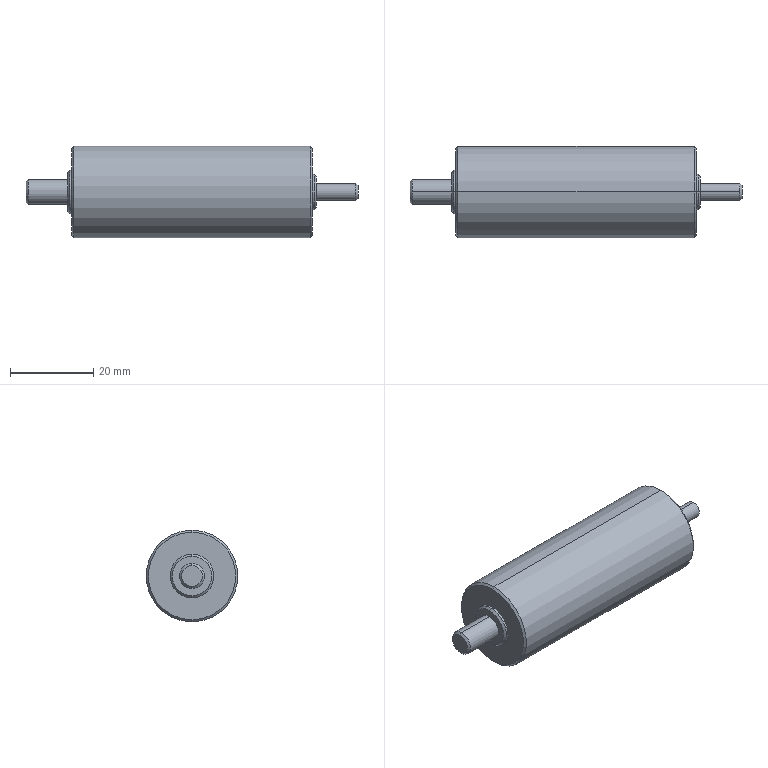Part | SolidWorks | features Chamfer 1, Revolution 1 | 1 solid | 28 faces | box 79.6 x 22 x 22 mm | volume 22421 mm3 | cone 12 | cylinder 10 | plane 6 | commonest cylinder face diameters 4.024 x2 6 x2 8.524 x2 10.5 x2 22 x2
STEP:
#1=CARTESIAN_POINT('',(79.6,0.,-1.512));
#2=VERTEX_POINT('',#1);
#3=CARTESIAN_POINT('',(79.6,0.,1.512));
#4=VERTEX_POINT('',#3);
#5=CARTESIAN_POINT('',(79.6,0.,0.));
#6=DIRECTION('',(1.,0.,0.));
#7=DIRECTION('',(0.,0.,1.));
#8=AXIS2_PLACEMENT_3D('',#5,#6,#7);
#9=CIRCLE('',#8,1.512);
#10=EDGE_CURVE('',#2,#4,#9,.T.);
#11=ORIENTED_EDGE('',*,*,#10,.F.);
#12=CARTESIAN_POINT('',(79.1,0.,-2.012));
#13=VERTEX_POINT('',#12);
#14=CARTESIAN_POINT('',(79.1,0.,-2.012));
#15=DIRECTION('',(-0.7071,0.,-0.7071));
#16=VECTOR('',#15,1000.);
#17=LINE('',#14,#16);
#18=EDGE_CURVE('',#2,#13,#17,.T.);
#19=ORIENTED_EDGE('',*,*,#18,.T.);
#20=CARTESIAN_POINT('',(79.1,0.,2.012));
#21=VERTEX_POINT('',#20);
#22=CARTESIAN_POINT('',(79.1,0.,0.));
#23=DIRECTION('',(-1.,0.,0.));
#24=DIRECTION('',(0.,0.,1.));
#25=AXIS2_PLACEMENT_3D('',#22,#23,#24);
#26=CIRCLE('',#25,2.012);
#27=EDGE_CURVE('',#21,#13,#26,.T.);
#28=ORIENTED_EDGE('',*,*,#27,.F.);
#29=CARTESIAN_POINT('',(79.1,0.,2.012));
#30=DIRECTION('',(-0.7071,0.,0.7071));
#31=VECTOR('',#30,1000.);
#32=LINE('',#29,#31);
#33=EDGE_CURVE('',#4,#21,#32,.T.);
#34=ORIENTED_EDGE('',*,*,#33,.F.);
#35=EDGE_LOOP('',(#11,#19,#28,#34));
#36=FACE_OUTER_BOUND('',#35,.T.);
#37=CARTESIAN_POINT('',(79.1,0.,0.));
#38=DIRECTION('',(-1.,0.,0.));
#39=DIRECTION('',(0.,0.,1.));
#40=AXIS2_PLACEMENT_3D('',#37,#38,#39);
#41=CONICAL_SURFACE('',#40,2.012,0.7854);
#42=ADVANCED_FACE('',(#36),#41,.T.);
#43=CARTESIAN_POINT('',(69.6,0.,-3.762));
#44=VERTEX_POINT('',#43);
#45=CARTESIAN_POINT('',(69.6,0.,3.762));
#46=VERTEX_POINT('',#45);
#47=CARTESIAN_POINT('',(69.6,0.,0.));
#48=DIRECTION('',(1.,0.,0.));
#49=DIRECTION('',(0.,0.,1.));
#50=AXIS2_PLACEMENT_3D('',#47,#48,#49);
#51=CIRCLE('',#50,3.762);
#52=EDGE_CURVE('',#44,#46,#51,.T.);
#53=ORIENTED_EDGE('',*,*,#52,.F.);
#54=CARTESIAN_POINT('',(69.1,0.,-4.262));
#55=VERTEX_POINT('',#54);
#56=CARTESIAN_POINT('',(69.1,0.,-4.262));
#57=DIRECTION('',(-0.7071,0.,-0.7071));
#58=VECTOR('',#57,1000.);
#59=LINE('',#56,#58);
#60=EDGE_CURVE('',#44,#55,#59,.T.);
#61=ORIENTED_EDGE('',*,*,#60,.T.);
#62=CARTESIAN_POINT('',(69.1,0.,4.262));
#63=VERTEX_POINT('',#62);
#64=CARTESIAN_POINT('',(69.1,0.,0.));
#65=DIRECTION('',(-1.,0.,0.));
#66=DIRECTION('',(0.,0.,1.));
#67=AXIS2_PLACEMENT_3D('',#64,#65,#66);
#68=CIRCLE('',#67,4.262);
#69=EDGE_CURVE('',#63,#55,#68,.T.);
#70=ORIENTED_EDGE('',*,*,#69,.F.);
#71=CARTESIAN_POINT('',(69.1,0.,4.262));
#72=DIRECTION('',(-0.7071,0.,0.7071));
#73=VECTOR('',#72,1000.);
#74=LINE('',#71,#73);
#75=EDGE_CURVE('',#46,#63,#74,.T.);
#76=ORIENTED_EDGE('',*,*,#75,.F.);
#77=EDGE_LOOP('',(#53,#61,#70,#76));
#78=FACE_OUTER_BOUND('',#77,.T.);
#79=CARTESIAN_POINT('',(69.1,0.,0.));
#80=DIRECTION('',(-1.,0.,0.));
#81=DIRECTION('',(0.,0.,1.));
#82=AXIS2_PLACEMENT_3D('',#79,#80,#81);
#83=CONICAL_SURFACE('',#82,4.262,0.7854);
#84=ADVANCED_FACE('',(#78),#83,.T.);
#85=CARTESIAN_POINT('',(68.6,0.,-10.5));
#86=VERTEX_POINT('',#85);
#87=CARTESIAN_POINT('',(68.6,0.,10.5));
#88=VERTEX_POINT('',#87);
#89=CARTESIAN_POINT('',(68.6,0.,0.));
#90=DIRECTION('',(1.,0.,0.));
#91=DIRECTION('',(0.,0.,1.));
#92=AXIS2_PLACEMENT_3D('',#89,#90,#91);
#93=CIRCLE('',#92,10.5);
#94=EDGE_CURVE('',#86,#88,#93,.T.);
#95=ORIENTED_EDGE('',*,*,#94,.F.);
#96=CARTESIAN_POINT('',(68.1,0.,-11.));
#97=VERTEX_POINT('',#96);
#98=CARTESIAN_POINT('',(68.1,0.,-11.));
#99=DIRECTION('',(-0.7071,0.,-0.7071));
#100=VECTOR('',#99,1000.);
#101=LINE('',#98,#100);
#102=EDGE_CURVE('',#86,#97,#101,.T.);
#103=ORIENTED_EDGE('',*,*,#102,.T.);
#104=CARTESIAN_POINT('',(68.1,0.,11.));
#105=VERTEX_POINT('',#104);
#106=CARTESIAN_POINT('',(68.1,0.,0.));
#107=DIRECTION('',(-1.,0.,0.));
#108=DIRECTION('',(0.,0.,1.));
#109=AXIS2_PLACEMENT_3D('',#106,#107,#108);
#110=CIRCLE('',#109,11.);
#111=EDGE_CURVE('',#105,#97,#110,.T.);
#112=ORIENTED_EDGE('',*,*,#111,.F.);
#113=CARTESIAN_POINT('',(68.1,0.,11.));
#114=DIRECTION('',(-0.7071,0.,0.7071));
#115=VECTOR('',#114,1000.);
#116=LINE('',#113,#115);
#117=EDGE_CURVE('',#88,#105,#116,.T.);
#118=ORIENTED_EDGE('',*,*,#117,.F.);
#119=EDGE_LOOP('',(#95,#103,#112,#118));
#120=FACE_OUTER_BOUND('',#119,.T.);
#121=CARTESIAN_POINT('',(68.1,0.,0.));
#122=DIRECTION('',(-1.,0.,0.));
#123=DIRECTION('',(0.,0.,1.));
#124=AXIS2_PLACEMENT_3D('',#121,#122,#123);
#125=CONICAL_SURFACE('',#124,11.,0.7854);
#126=ADVANCED_FACE('',(#120),#125,.T.);
#127=CARTESIAN_POINT('',(11.,0.,10.5));
#128=VERTEX_POINT('',#127);
#129=CARTESIAN_POINT('',(11.,0.,-10.5));
#130=VERTEX_POINT('',#129);
#131=CARTESIAN_POINT('',(11.,0.,0.));
#132=DIRECTION('',(-1.,0.,0.));
#133=DIRECTION('',(0.,0.,-1.));
#134=AXIS2_PLACEMENT_3D('',#131,#132,#133);
#135=CIRCLE('',#134,10.5);
#136=EDGE_CURVE('',#128,#130,#135,.T.);
#137=ORIENTED_EDGE('',*,*,#136,.F.);
#138=CARTESIAN_POINT('',(11.5,0.,11.));
#139=VERTEX_POINT('',#138);
#140=CARTESIAN_POINT('',(11.,0.,10.5));
#141=DIRECTION('',(0.7071,0.,0.7071));
#142=VECTOR('',#141,1000.);
#143=LINE('',#140,#142);
#144=EDGE_CURVE('',#128,#139,#143,.T.);
#145=ORIENTED_EDGE('',*,*,#144,.T.);
#146=CARTESIAN_POINT('',(11.5,0.,-11.));
#147=VERTEX_POINT('',#146);
#148=CARTESIAN_POINT('',(11.5,0.,0.));
#149=DIRECTION('',(1.,0.,0.));
#150=DIRECTION('',(0.,0.,-1.));
#151=AXIS2_PLACEMENT_3D('',#148,#149,#150);
#152=CIRCLE('',#151,11.);
#153=EDGE_CURVE('',#147,#139,#152,.T.);
#154=ORIENTED_EDGE('',*,*,#153,.F.);
#155=CARTESIAN_POINT('',(11.,0.,-10.5));
#156=DIRECTION('',(0.7071,0.,-0.7071));
#157=VECTOR('',#156,1000.);
#158=LINE('',#155,#157);
#159=EDGE_CURVE('',#130,#147,#158,.T.);
#160=ORIENTED_EDGE('',*,*,#159,.F.);
#161=EDGE_LOOP('',(#137,#145,#154,#160));
#162=FACE_OUTER_BOUND('',#161,.T.);
#163=CARTESIAN_POINT('',(11.,0.,0.));
#164=DIRECTION('',(1.,0.,0.));
#165=DIRECTION('',(0.,0.,-1.));
#166=AXIS2_PLACEMENT_3D('',#163,#164,#165);
#167=CONICAL_SURFACE('',#166,10.5,0.7854);
#168=ADVANCED_FACE('',(#162),#167,.T.);
#169=CARTESIAN_POINT('',(10.,0.,4.75));
#170=VERTEX_POINT('',#169);
#171=CARTESIAN_POINT('',(10.,0.,-4.75));
#172=VERTEX_POINT('',#171);
#173=CARTESIAN_POINT('',(10.,0.,0.));
#174=DIRECTION('',(-1.,0.,0.));
#175=DIRECTION('',(0.,0.,-1.));
#176=AXIS2_PLACEMENT_3D('',#173,#174,#175);
#177=CIRCLE('',#176,4.75);
#178=EDGE_CURVE('',#170,#172,#177,.T.);
#179=ORIENTED_EDGE('',*,*,#178,.F.);
#180=CARTESIAN_POINT('',(10.5,0.,5.25));
#181=VERTEX_POINT('',#180);
#182=CARTESIAN_POINT('',(10.,0.,4.75));
#183=DIRECTION('',(0.7071,0.,0.7071));
#184=VECTOR('',#183,1000.);
#185=LINE('',#182,#184);
#186=EDGE_CURVE('',#170,#181,#185,.T.);
#187=ORIENTED_EDGE('',*,*,#186,.T.);
#188=CARTESIAN_POINT('',(10.5,0.,-5.25));
#189=VERTEX_POINT('',#188);
#190=CARTESIAN_POINT('',(10.5,0.,0.));
#191=DIRECTION('',(1.,0.,0.));
#192=DIRECTION('',(0.,0.,-1.));
#193=AXIS2_PLACEMENT_3D('',#190,#191,#192);
#194=CIRCLE('',#193,5.25);
#195=EDGE_CURVE('',#189,#181,#194,.T.);
#196=ORIENTED_EDGE('',*,*,#195,.F.);
#197=CARTESIAN_POINT('',(10.,0.,-4.75));
#198=DIRECTION('',(0.7071,0.,-0.7071));
#199=VECTOR('',#198,1000.);
#200=LINE('',#197,#199);
#201=EDGE_CURVE('',#172,#189,#200,.T.);
#202=ORIENTED_EDGE('',*,*,#201,.F.);
#203=EDGE_LOOP('',(#179,#187,#196,#202));
#204=FACE_OUTER_BOUND('',#203,.T.);
#205=CARTESIAN_POINT('',(10.,0.,0.));
#206=DIRECTION('',(1.,0.,0.));
#207=DIRECTION('',(0.,0.,-1.));
#208=AXIS2_PLACEMENT_3D('',#205,#206,#207);
#209=CONICAL_SURFACE('',#208,4.75,0.7854);
#210=ADVANCED_FACE('',(#204),#209,.T.);
#211=CARTESIAN_POINT('',(0.,0.,2.5));
#212=VERTEX_POINT('',#211);
#213=CARTESIAN_POINT('',(0.,0.,-2.5));
#214=VERTEX_POINT('',#213);
#215=CARTESIAN_POINT('',(0.,0.,0.));
#216=DIRECTION('',(-1.,0.,0.));
#217=DIRECTION('',(0.,0.,-1.));
#218=AXIS2_PLACEMENT_3D('',#215,#216,#217);
#219=CIRCLE('',#218,2.5);
#220=EDGE_CURVE('',#212,#214,#219,.T.);
#221=ORIENTED_EDGE('',*,*,#220,.F.);
#222=CARTESIAN_POINT('',(0.5,0.,3.));
#223=VERTEX_POINT('',#222);
#224=CARTESIAN_POINT('',(0.,0.,2.5));
#225=DIRECTION('',(0.7071,0.,0.7071));
#226=VECTOR('',#225,1000.);
#227=LINE('',#224,#226);
#228=EDGE_CURVE('',#212,#223,#227,.T.);
#229=ORIENTED_EDGE('',*,*,#228,.T.);
#230=CARTESIAN_POINT('',(0.5,0.,-3.));
#231=VERTEX_POINT('',#230);
#232=CARTESIAN_POINT('',(0.5,0.,0.));
#233=DIRECTION('',(1.,0.,0.));
#234=DIRECTION('',(0.,0.,-1.));
#235=AXIS2_PLACEMENT_3D('',#232,#233,#234);
#236=CIRCLE('',#235,3.);
#237=EDGE_CURVE('',#231,#223,#236,.T.);
#238=ORIENTED_EDGE('',*,*,#237,.F.);
#239=CARTESIAN_POINT('',(0.,0.,-2.5));
#240=DIRECTION('',(0.7071,0.,-0.7071));
#241=VECTOR('',#240,1000.);
#242=LINE('',#239,#241);
#243=EDGE_CURVE('',#214,#231,#242,.T.);
#244=ORIENTED_EDGE('',*,*,#243,.F.);
#245=EDGE_LOOP('',(#221,#229,#238,#244));
#246=FACE_OUTER_BOUND('',#245,.T.);
#247=CARTESIAN_POINT('',(0.,0.,0.));
#248=DIRECTION('',(1.,0.,0.));
#249=DIRECTION('',(0.,0.,-1.));
#250=AXIS2_PLACEMENT_3D('',#247,#248,#249);
#251=CONICAL_SURFACE('',#250,2.5,0.7854);
#252=ADVANCED_FACE('',(#246),#251,.T.);
#253=ORIENTED_EDGE('',*,*,#27,.T.);
#254=CARTESIAN_POINT('',(69.6,0.,-2.012));
#255=VERTEX_POINT('',#254);
#256=CARTESIAN_POINT('',(0.,0.,-2.012));
#257=DIRECTION('',(-1.,0.,0.));
#258=VECTOR('',#257,1000.);
#259=LINE('',#256,#258);
#260=EDGE_CURVE('',#13,#255,#259,.T.);
#261=ORIENTED_EDGE('',*,*,#260,.T.);
#262=CARTESIAN_POINT('',(69.6,0.,2.012));
#263=VERTEX_POINT('',#262);
#264=CARTESIAN_POINT('',(69.6,0.,0.));
#265=DIRECTION('',(-1.,0.,0.));
#266=DIRECTION('',(0.,0.,1.));
#267=AXIS2_PLACEMENT_3D('',#264,#265,#266);
#268=CIRCLE('',#267,2.012);
#269=EDGE_CURVE('',#263,#255,#268,.T.);
#270=ORIENTED_EDGE('',*,*,#269,.F.);
#271=CARTESIAN_POINT('',(0.,0.,2.012));
#272=DIRECTION('',(-1.,0.,0.));
#273=VECTOR('',#272,1000.);
#274=LINE('',#271,#273);
#275=EDGE_CURVE('',#21,#263,#274,.T.);
#276=ORIENTED_EDGE('',*,*,#275,.F.);
#277=EDGE_LOOP('',(#253,#261,#270,#276));
#278=FACE_OUTER_BOUND('',#277,.T.);
#279=CARTESIAN_POINT('',(0.,0.,0.));
#280=DIRECTION('',(-1.,0.,0.));
#281=DIRECTION('',(0.,0.,1.));
#282=AXIS2_PLACEMENT_3D('',#279,#280,#281);
#283=CYLINDRICAL_SURFACE('',#282,2.012);
#284=ADVANCED_FACE('',(#278),#283,.T.);
#285=ORIENTED_EDGE('',*,*,#69,.T.);
#286=CARTESIAN_POINT('',(68.6,0.,-4.262));
#287=VERTEX_POINT('',#286);
#288=CARTESIAN_POINT('',(0.,0.,-4.262));
#289=DIRECTION('',(-1.,0.,0.));
#290=VECTOR('',#289,1000.);
#291=LINE('',#288,#290);
#292=EDGE_CURVE('',#55,#287,#291,.T.);
#293=ORIENTED_EDGE('',*,*,#292,.T.);
#294=CARTESIAN_POINT('',(68.6,0.,4.262));
#295=VERTEX_POINT('',#294);
#296=CARTESIAN_POINT('',(68.6,0.,0.));
#297=DIRECTION('',(-1.,0.,0.));
#298=DIRECTION('',(0.,0.,1.));
#299=AXIS2_PLACEMENT_3D('',#296,#297,#298);
#300=CIRCLE('',#299,4.262);
#301=EDGE_CURVE('',#295,#287,#300,.T.);
#302=ORIENTED_EDGE('',*,*,#301,.F.);
#303=CARTESIAN_POINT('',(0.,0.,4.262));
#304=DIRECTION('',(-1.,0.,0.));
#305=VECTOR('',#304,1000.);
#306=LINE('',#303,#305);
#307=EDGE_CURVE('',#63,#295,#306,.T.);
#308=ORIENTED_EDGE('',*,*,#307,.F.);
#309=EDGE_LOOP('',(#285,#293,#302,#308));
#310=FACE_OUTER_BOUND('',#309,.T.);
#311=CARTESIAN_POINT('',(0.,0.,0.));
#312=DIRECTION('',(-1.,0.,0.));
#313=DIRECTION('',(0.,0.,1.));
#314=AXIS2_PLACEMENT_3D('',#311,#312,#313);
#315=CYLINDRICAL_SURFACE('',#314,4.262);
#316=ADVANCED_FACE('',(#310),#315,.T.);
#317=ORIENTED_EDGE('',*,*,#111,.T.);
#318=CARTESIAN_POINT('',(0.,0.,-11.));
#319=DIRECTION('',(-1.,0.,0.));
#320=VECTOR('',#319,1000.);
#321=LINE('',#318,#320);
#322=EDGE_CURVE('',#97,#147,#321,.T.);
#323=ORIENTED_EDGE('',*,*,#322,.T.);
#324=ORIENTED_EDGE('',*,*,#153,.T.);
#325=CARTESIAN_POINT('',(0.,0.,11.));
#326=DIRECTION('',(-1.,0.,0.));
#327=VECTOR('',#326,1000.);
#328=LINE('',#325,#327);
#329=EDGE_CURVE('',#105,#139,#328,.T.);
#330=ORIENTED_EDGE('',*,*,#329,.F.);
#331=EDGE_LOOP('',(#317,#323,#324,#330));
#332=FACE_OUTER_BOUND('',#331,.T.);
#333=CARTESIAN_POINT('',(0.,0.,0.));
#334=DIRECTION('',(-1.,0.,0.));
#335=DIRECTION('',(0.,0.,1.));
#336=AXIS2_PLACEMENT_3D('',#333,#334,#335);
#337=CYLINDRICAL_SURFACE('',#336,11.);
#338=ADVANCED_FACE('',(#332),#337,.T.);
#339=CARTESIAN_POINT('',(11.,0.,5.25));
#340=VERTEX_POINT('',#339);
#341=CARTESIAN_POINT('',(11.,0.,-5.25));
#342=VERTEX_POINT('',#341);
#343=CARTESIAN_POINT('',(11.,0.,0.));
#344=DIRECTION('',(-1.,0.,0.));
#345=DIRECTION('',(0.,0.,1.));
#346=AXIS2_PLACEMENT_3D('',#343,#344,#345);
#347=CIRCLE('',#346,5.25);
#348=EDGE_CURVE('',#340,#342,#347,.T.);
#349=ORIENTED_EDGE('',*,*,#348,.T.);
#350=CARTESIAN_POINT('',(0.,0.,-5.25));
#351=DIRECTION('',(-1.,0.,0.));
#352=VECTOR('',#351,1000.);
#353=LINE('',#350,#352);
#354=EDGE_CURVE('',#342,#189,#353,.T.);
#355=ORIENTED_EDGE('',*,*,#354,.T.);
#356=ORIENTED_EDGE('',*,*,#195,.T.);
#357=CARTESIAN_POINT('',(0.,0.,5.25));
#358=DIRECTION('',(-1.,0.,0.));
#359=VECTOR('',#358,1000.);
#360=LINE('',#357,#359);
#361=EDGE_CURVE('',#340,#181,#360,.T.);
#362=ORIENTED_EDGE('',*,*,#361,.F.);
#363=EDGE_LOOP('',(#349,#355,#356,#362));
#364=FACE_OUTER_BOUND('',#363,.T.);
#365=CARTESIAN_POINT('',(0.,0.,0.));
#366=DIRECTION('',(-1.,0.,0.));
#367=DIRECTION('',(0.,0.,1.));
#368=AXIS2_PLACEMENT_3D('',#365,#366,#367);
#369=CYLINDRICAL_SURFACE('',#368,5.25);
#370=ADVANCED_FACE('',(#364),#369,.T.);
#371=CARTESIAN_POINT('',(10.,0.,3.));
#372=VERTEX_POINT('',#371);
#373=CARTESIAN_POINT('',(10.,0.,-3.));
#374=VERTEX_POINT('',#373);
#375=CARTESIAN_POINT('',(10.,0.,0.));
#376=DIRECTION('',(-1.,0.,0.));
#377=DIRECTION('',(0.,0.,1.));
#378=AXIS2_PLACEMENT_3D('',#375,#376,#377);
#379=CIRCLE('',#378,3.);
#380=EDGE_CURVE('',#372,#374,#379,.T.);
#381=ORIENTED_EDGE('',*,*,#380,.T.);
#382=CARTESIAN_POINT('',(0.,0.,-3.));
#383=DIRECTION('',(-1.,0.,0.));
#384=VECTOR('',#383,1000.);
#385=LINE('',#382,#384);
#386=EDGE_CURVE('',#374,#231,#385,.T.);
#387=ORIENTED_EDGE('',*,*,#386,.T.);
#388=ORIENTED_EDGE('',*,*,#237,.T.);
#389=CARTESIAN_POINT('',(0.,0.,3.));
#390=DIRECTION('',(-1.,0.,0.));
#391=VECTOR('',#390,1000.);
#392=LINE('',#389,#391);
#393=EDGE_CURVE('',#372,#223,#392,.T.);
#394=ORIENTED_EDGE('',*,*,#393,.F.);
#395=EDGE_LOOP('',(#381,#387,#388,#394));
#396=FACE_OUTER_BOUND('',#395,.T.);
#397=CARTESIAN_POINT('',(0.,0.,0.));
#398=DIRECTION('',(-1.,0.,0.));
#399=DIRECTION('',(0.,0.,1.));
#400=AXIS2_PLACEMENT_3D('',#397,#398,#399);
#401=CYLINDRICAL_SURFACE('',#400,3.);
#402=ADVANCED_FACE('',(#396),#401,.T.);
#403=CARTESIAN_POINT('',(0.,0.,0.));
#404=DIRECTION('',(-1.,0.,0.));
#405=DIRECTION('',(0.,0.,-1.));
#406=AXIS2_PLACEMENT_3D('',#403,#404,#405);
#407=CIRCLE('',#406,2.5);
#408=EDGE_CURVE('',#214,#212,#407,.T.);
#409=ORIENTED_EDGE('',*,*,#408,.T.);
#410=ORIENTED_EDGE('',*,*,#220,.T.);
#411=EDGE_LOOP('',(#409,#410));
#412=FACE_OUTER_BOUND('',#411,.T.);
#413=CARTESIAN_POINT('',(0.,0.,0.));
#414=DIRECTION('',(1.,0.,0.));
#415=DIRECTION('',(0.,0.,-1.));
#416=AXIS2_PLACEMENT_3D('',#413,#414,#415);
#417=PLANE('',#416);
#418=ADVANCED_FACE('',(#412),#417,.F.);
#419=ORIENTED_EDGE('',*,*,#386,.F.);
#420=CARTESIAN_POINT('',(10.,0.,0.));
#421=DIRECTION('',(-1.,0.,0.));
#422=DIRECTION('',(0.,0.,1.));
#423=AXIS2_PLACEMENT_3D('',#420,#421,#422);
#424=CIRCLE('',#423,3.);
#425=EDGE_CURVE('',#374,#372,#424,.T.);
#426=ORIENTED_EDGE('',*,*,#425,.T.);
#427=ORIENTED_EDGE('',*,*,#393,.T.);
#428=CARTESIAN_POINT('',(0.5,0.,0.));
#429=DIRECTION('',(1.,0.,0.));
#430=DIRECTION('',(0.,0.,-1.));
#431=AXIS2_PLACEMENT_3D('',#428,#429,#430);
#432=CIRCLE('',#431,3.);
#433=EDGE_CURVE('',#223,#231,#432,.T.);
#434=ORIENTED_EDGE('',*,*,#433,.T.);
#435=EDGE_LOOP('',(#419,#426,#427,#434));
#436=FACE_OUTER_BOUND('',#435,.T.);
#437=CARTESIAN_POINT('',(0.,0.,0.));
#438=DIRECTION('',(-1.,0.,0.));
#439=DIRECTION('',(0.,0.,1.));
#440=AXIS2_PLACEMENT_3D('',#437,#438,#439);
#441=CYLINDRICAL_SURFACE('',#440,3.);
#442=ADVANCED_FACE('',(#436),#441,.T.);
#443=CARTESIAN_POINT('',(10.,0.,0.));
#444=DIRECTION('',(-1.,0.,0.));
#445=DIRECTION('',(0.,0.,-1.));
#446=AXIS2_PLACEMENT_3D('',#443,#444,#445);
#447=CIRCLE('',#446,4.75);
#448=EDGE_CURVE('',#172,#170,#447,.T.);
#449=ORIENTED_EDGE('',*,*,#448,.T.);
#450=ORIENTED_EDGE('',*,*,#178,.T.);
#451=EDGE_LOOP('',(#449,#450));
#452=FACE_OUTER_BOUND('',#451,.T.);
#453=ORIENTED_EDGE('',*,*,#380,.F.);
#454=ORIENTED_EDGE('',*,*,#425,.F.);
#455=EDGE_LOOP('',(#453,#454));
#456=FACE_BOUND('',#455,.T.);
#457=CARTESIAN_POINT('',(10.,3.,0.));
#458=DIRECTION('',(1.,0.,0.));
#459=DIRECTION('',(0.,0.,-1.));
#460=AXIS2_PLACEMENT_3D('',#457,#458,#459);
#461=PLANE('',#460);
#462=ADVANCED_FACE('',(#452,#456),#461,.F.);
#463=ORIENTED_EDGE('',*,*,#354,.F.);
#464=CARTESIAN_POINT('',(11.,0.,0.));
#465=DIRECTION('',(-1.,0.,0.));
#466=DIRECTION('',(0.,0.,1.));
#467=AXIS2_PLACEMENT_3D('',#464,#465,#466);
#468=CIRCLE('',#467,5.25);
#469=EDGE_CURVE('',#342,#340,#468,.T.);
#470=ORIENTED_EDGE('',*,*,#469,.T.);
#471=ORIENTED_EDGE('',*,*,#361,.T.);
#472=CARTESIAN_POINT('',(10.5,0.,0.));
#473=DIRECTION('',(1.,0.,0.));
#474=DIRECTION('',(0.,0.,-1.));
#475=AXIS2_PLACEMENT_3D('',#472,#473,#474);
#476=CIRCLE('',#475,5.25);
#477=EDGE_CURVE('',#181,#189,#476,.T.);
#478=ORIENTED_EDGE('',*,*,#477,.T.);
#479=EDGE_LOOP('',(#463,#470,#471,#478));
#480=FACE_OUTER_BOUND('',#479,.T.);
#481=CARTESIAN_POINT('',(0.,0.,0.));
#482=DIRECTION('',(-1.,0.,0.));
#483=DIRECTION('',(0.,0.,1.));
#484=AXIS2_PLACEMENT_3D('',#481,#482,#483);
#485=CYLINDRICAL_SURFACE('',#484,5.25);
#486=ADVANCED_FACE('',(#480),#485,.T.);
#487=CARTESIAN_POINT('',(11.,0.,0.));
#488=DIRECTION('',(-1.,0.,0.));
#489=DIRECTION('',(0.,0.,-1.));
#490=AXIS2_PLACEMENT_3D('',#487,#488,#489);
#491=CIRCLE('',#490,10.5);
#492=EDGE_CURVE('',#130,#128,#491,.T.);
#493=ORIENTED_EDGE('',*,*,#492,.T.);
#494=ORIENTED_EDGE('',*,*,#136,.T.);
#495=EDGE_LOOP('',(#493,#494));
#496=FACE_OUTER_BOUND('',#495,.T.);
#497=ORIENTED_EDGE('',*,*,#348,.F.);
#498=ORIENTED_EDGE('',*,*,#469,.F.);
#499=EDGE_LOOP('',(#497,#498));
#500=FACE_BOUND('',#499,.T.);
#501=CARTESIAN_POINT('',(11.,5.25,0.));
#502=DIRECTION('',(1.,0.,0.));
#503=DIRECTION('',(0.,0.,-1.));
#504=AXIS2_PLACEMENT_3D('',#501,#502,#503);
#505=PLANE('',#504);
#506=ADVANCED_FACE('',(#496,#500),#505,.F.);
#507=ORIENTED_EDGE('',*,*,#322,.F.);
#508=CARTESIAN_POINT('',(68.1,0.,0.));
#509=DIRECTION('',(-1.,0.,0.));
#510=DIRECTION('',(0.,0.,1.));
#511=AXIS2_PLACEMENT_3D('',#508,#509,#510);
#512=CIRCLE('',#511,11.);
#513=EDGE_CURVE('',#97,#105,#512,.T.);
#514=ORIENTED_EDGE('',*,*,#513,.T.);
#515=ORIENTED_EDGE('',*,*,#329,.T.);
#516=CARTESIAN_POINT('',(11.5,0.,0.));
#517=DIRECTION('',(1.,0.,0.));
#518=DIRECTION('',(0.,0.,-1.));
#519=AXIS2_PLACEMENT_3D('',#516,#517,#518);
#520=CIRCLE('',#519,11.);
#521=EDGE_CURVE('',#139,#147,#520,.T.);
#522=ORIENTED_EDGE('',*,*,#521,.T.);
#523=EDGE_LOOP('',(#507,#514,#515,#522));
#524=FACE_OUTER_BOUND('',#523,.T.);
#525=CARTESIAN_POINT('',(0.,0.,0.));
#526=DIRECTION('',(-1.,0.,0.));
#527=DIRECTION('',(0.,0.,1.));
#528=AXIS2_PLACEMENT_3D('',#525,#526,#527);
#529=CYLINDRICAL_SURFACE('',#528,11.);
#530=ADVANCED_FACE('',(#524),#529,.T.);
#531=CARTESIAN_POINT('',(68.6,0.,0.));
#532=DIRECTION('',(1.,0.,0.));
#533=DIRECTION('',(0.,0.,1.));
#534=AXIS2_PLACEMENT_3D('',#531,#532,#533);
#535=CIRCLE('',#534,10.5);
#536=EDGE_CURVE('',#88,#86,#535,.T.);
#537=ORIENTED_EDGE('',*,*,#536,.T.);
#538=ORIENTED_EDGE('',*,*,#94,.T.);
#539=EDGE_LOOP('',(#537,#538));
#540=FACE_OUTER_BOUND('',#539,.T.);
#541=ORIENTED_EDGE('',*,*,#301,.T.);
#542=CARTESIAN_POINT('',(68.6,0.,0.));
#543=DIRECTION('',(-1.,0.,0.));
#544=DIRECTION('',(0.,0.,1.));
#545=AXIS2_PLACEMENT_3D('',#542,#543,#544);
#546=CIRCLE('',#545,4.262);
#547=EDGE_CURVE('',#287,#295,#546,.T.);
#548=ORIENTED_EDGE('',*,*,#547,.T.);
#549=EDGE_LOOP('',(#541,#548));
#550=FACE_BOUND('',#549,.T.);
#551=CARTESIAN_POINT('',(68.6,11.,0.));
#552=DIRECTION('',(-1.,0.,0.));
#553=DIRECTION('',(0.,0.,1.));
#554=AXIS2_PLACEMENT_3D('',#551,#552,#553);
#555=PLANE('',#554);
#556=ADVANCED_FACE('',(#540,#550),#555,.F.);
#557=ORIENTED_EDGE('',*,*,#292,.F.);
#558=CARTESIAN_POINT('',(69.1,0.,0.));
#559=DIRECTION('',(-1.,0.,0.));
#560=DIRECTION('',(0.,0.,1.));
#561=AXIS2_PLACEMENT_3D('',#558,#559,#560);
#562=CIRCLE('',#561,4.262);
#563=EDGE_CURVE('',#55,#63,#562,.T.);
#564=ORIENTED_EDGE('',*,*,#563,.T.);
#565=ORIENTED_EDGE('',*,*,#307,.T.);
#566=ORIENTED_EDGE('',*,*,#547,.F.);
#567=EDGE_LOOP('',(#557,#564,#565,#566));
#568=FACE_OUTER_BOUND('',#567,.T.);
#569=CARTESIAN_POINT('',(0.,0.,0.));
#570=DIRECTION('',(-1.,0.,0.));
#571=DIRECTION('',(0.,0.,1.));
#572=AXIS2_PLACEMENT_3D('',#569,#570,#571);
#573=CYLINDRICAL_SURFACE('',#572,4.262);
#574=ADVANCED_FACE('',(#568),#573,.T.);
#575=CARTESIAN_POINT('',(69.6,0.,0.));
#576=DIRECTION('',(1.,0.,0.));
#577=DIRECTION('',(0.,0.,1.));
#578=AXIS2_PLACEMENT_3D('',#575,#576,#577);
#579=CIRCLE('',#578,3.762);
#580=EDGE_CURVE('',#46,#44,#579,.T.);
#581=ORIENTED_EDGE('',*,*,#580,.T.);
#582=ORIENTED_EDGE('',*,*,#52,.T.);
#583=EDGE_LOOP('',(#581,#582));
#584=FACE_OUTER_BOUND('',#583,.T.);
#585=ORIENTED_EDGE('',*,*,#269,.T.);
#586=CARTESIAN_POINT('',(69.6,0.,0.));
#587=DIRECTION('',(-1.,0.,0.));
#588=DIRECTION('',(0.,0.,1.));
#589=AXIS2_PLACEMENT_3D('',#586,#587,#588);
#590=CIRCLE('',#589,2.012);
#591=EDGE_CURVE('',#255,#263,#590,.T.);
#592=ORIENTED_EDGE('',*,*,#591,.T.);
#593=EDGE_LOOP('',(#585,#592));
#594=FACE_BOUND('',#593,.T.);
#595=CARTESIAN_POINT('',(69.6,4.262,0.));
#596=DIRECTION('',(-1.,0.,0.));
#597=DIRECTION('',(0.,0.,1.));
#598=AXIS2_PLACEMENT_3D('',#595,#596,#597);
#599=PLANE('',#598);
#600=ADVANCED_FACE('',(#584,#594),#599,.F.);
#601=ORIENTED_EDGE('',*,*,#260,.F.);
#602=CARTESIAN_POINT('',(79.1,0.,0.));
#603=DIRECTION('',(-1.,0.,0.));
#604=DIRECTION('',(0.,0.,1.));
#605=AXIS2_PLACEMENT_3D('',#602,#603,#604);
#606=CIRCLE('',#605,2.012);
#607=EDGE_CURVE('',#13,#21,#606,.T.);
#608=ORIENTED_EDGE('',*,*,#607,.T.);
#609=ORIENTED_EDGE('',*,*,#275,.T.);
#610=ORIENTED_EDGE('',*,*,#591,.F.);
#611=EDGE_LOOP('',(#601,#608,#609,#610));
#612=FACE_OUTER_BOUND('',#611,.T.);
#613=CARTESIAN_POINT('',(0.,0.,0.));
#614=DIRECTION('',(-1.,0.,0.));
#615=DIRECTION('',(0.,0.,1.));
#616=AXIS2_PLACEMENT_3D('',#613,#614,#615);
#617=CYLINDRICAL_SURFACE('',#616,2.012);
#618=ADVANCED_FACE('',(#612),#617,.T.);
#619=CARTESIAN_POINT('',(79.6,0.,0.));
#620=DIRECTION('',(1.,0.,0.));
#621=DIRECTION('',(0.,0.,1.));
#622=AXIS2_PLACEMENT_3D('',#619,#620,#621);
#623=CIRCLE('',#622,1.512);
#624=EDGE_CURVE('',#4,#2,#623,.T.);
#625=ORIENTED_EDGE('',*,*,#624,.T.);
#626=ORIENTED_EDGE('',*,*,#10,.T.);
#627=EDGE_LOOP('',(#625,#626));
#628=FACE_OUTER_BOUND('',#627,.T.);
#629=CARTESIAN_POINT('',(79.6,2.012,0.));
#630=DIRECTION('',(-1.,0.,0.));
#631=DIRECTION('',(0.,0.,1.));
#632=AXIS2_PLACEMENT_3D('',#629,#630,#631);
#633=PLANE('',#632);
#634=ADVANCED_FACE('',(#628),#633,.F.);
#635=ORIENTED_EDGE('',*,*,#228,.F.);
#636=ORIENTED_EDGE('',*,*,#408,.F.);
#637=ORIENTED_EDGE('',*,*,#243,.T.);
#638=ORIENTED_EDGE('',*,*,#433,.F.);
#639=EDGE_LOOP('',(#635,#636,#637,#638));
#640=FACE_OUTER_BOUND('',#639,.T.);
#641=CARTESIAN_POINT('',(0.,0.,0.));
#642=DIRECTION('',(1.,0.,0.));
#643=DIRECTION('',(0.,0.,-1.));
#644=AXIS2_PLACEMENT_3D('',#641,#642,#643);
#645=CONICAL_SURFACE('',#644,2.5,0.7854);
#646=ADVANCED_FACE('',(#640),#645,.T.);
#647=ORIENTED_EDGE('',*,*,#186,.F.);
#648=ORIENTED_EDGE('',*,*,#448,.F.);
#649=ORIENTED_EDGE('',*,*,#201,.T.);
#650=ORIENTED_EDGE('',*,*,#477,.F.);
#651=EDGE_LOOP('',(#647,#648,#649,#650));
#652=FACE_OUTER_BOUND('',#651,.T.);
#653=CARTESIAN_POINT('',(10.,0.,0.));
#654=DIRECTION('',(1.,0.,0.));
#655=DIRECTION('',(0.,0.,-1.));
#656=AXIS2_PLACEMENT_3D('',#653,#654,#655);
#657=CONICAL_SURFACE('',#656,4.75,0.7854);
#658=ADVANCED_FACE('',(#652),#657,.T.);
#659=ORIENTED_EDGE('',*,*,#144,.F.);
#660=ORIENTED_EDGE('',*,*,#492,.F.);
#661=ORIENTED_EDGE('',*,*,#159,.T.);
#662=ORIENTED_EDGE('',*,*,#521,.F.);
#663=EDGE_LOOP('',(#659,#660,#661,#662));
#664=FACE_OUTER_BOUND('',#663,.T.);
#665=CARTESIAN_POINT('',(11.,0.,0.));
#666=DIRECTION('',(1.,0.,0.));
#667=DIRECTION('',(0.,0.,-1.));
#668=AXIS2_PLACEMENT_3D('',#665,#666,#667);
#669=CONICAL_SURFACE('',#668,10.5,0.7854);
#670=ADVANCED_FACE('',(#664),#669,.T.);
#671=ORIENTED_EDGE('',*,*,#102,.F.);
#672=ORIENTED_EDGE('',*,*,#536,.F.);
#673=ORIENTED_EDGE('',*,*,#117,.T.);
#674=ORIENTED_EDGE('',*,*,#513,.F.);
#675=EDGE_LOOP('',(#671,#672,#673,#674));
#676=FACE_OUTER_BOUND('',#675,.T.);
#677=CARTESIAN_POINT('',(68.1,0.,0.));
#678=DIRECTION('',(-1.,0.,0.));
#679=DIRECTION('',(0.,0.,1.));
#680=AXIS2_PLACEMENT_3D('',#677,#678,#679);
#681=CONICAL_SURFACE('',#680,11.,0.7854);
#682=ADVANCED_FACE('',(#676),#681,.T.);
#683=ORIENTED_EDGE('',*,*,#60,.F.);
#684=ORIENTED_EDGE('',*,*,#580,.F.);
#685=ORIENTED_EDGE('',*,*,#75,.T.);
#686=ORIENTED_EDGE('',*,*,#563,.F.);
#687=EDGE_LOOP('',(#683,#684,#685,#686));
#688=FACE_OUTER_BOUND('',#687,.T.);
#689=CARTESIAN_POINT('',(69.1,0.,0.));
#690=DIRECTION('',(-1.,0.,0.));
#691=DIRECTION('',(0.,0.,1.));
#692=AXIS2_PLACEMENT_3D('',#689,#690,#691);
#693=CONICAL_SURFACE('',#692,4.262,0.7854);
#694=ADVANCED_FACE('',(#688),#693,.T.);
#695=ORIENTED_EDGE('',*,*,#18,.F.);
#696=ORIENTED_EDGE('',*,*,#624,.F.);
#697=ORIENTED_EDGE('',*,*,#33,.T.);
#698=ORIENTED_EDGE('',*,*,#607,.F.);
#699=EDGE_LOOP('',(#695,#696,#697,#698));
#700=FACE_OUTER_BOUND('',#699,.T.);
#701=CARTESIAN_POINT('',(79.1,0.,0.));
#702=DIRECTION('',(-1.,0.,0.));
#703=DIRECTION('',(0.,0.,1.));
#704=AXIS2_PLACEMENT_3D('',#701,#702,#703);
#705=CONICAL_SURFACE('',#704,2.012,0.7854);
#706=ADVANCED_FACE('',(#700),#705,.T.);
#707=CLOSED_SHELL('',(#42,#84,#126,#168,#210,#252,#284,#316,#338,#370,#402,#418,#442,#462,#486,#506,#530,#556,#574,#600,#618,#634,#646,#658,#670,#682,#694,#706));
#708=MANIFOLD_SOLID_BREP('',#707);
#709=CARTESIAN_POINT('',(0.,0.,0.));
#710=DIRECTION('',(0.,0.,1.));
#711=DIRECTION('',(1.,0.,0.));
#712=AXIS2_PLACEMENT_3D('',#709,#710,#711);
#713=(LENGTH_UNIT()NAMED_UNIT(*)SI_UNIT(.MILLI.,.METRE.));
#714=UNCERTAINTY_MEASURE_WITH_UNIT(LENGTH_MEASURE(0.00001),#713,'','');
#715=(NAMED_UNIT(*)PLANE_ANGLE_UNIT()SI_UNIT($,.RADIAN.));
#716=(NAMED_UNIT(*)SI_UNIT($,.STERADIAN.)SOLID_ANGLE_UNIT());
#717=(GEOMETRIC_REPRESENTATION_CONTEXT(3)GLOBAL_UNCERTAINTY_ASSIGNED_CONTEXT((#714))GLOBAL_UNIT_ASSIGNED_CONTEXT((#713,#715,#716))REPRESENTATION_CONTEXT('',''));
#718=ADVANCED_BREP_SHAPE_REPRESENTATION('',(#708,#712),#717);